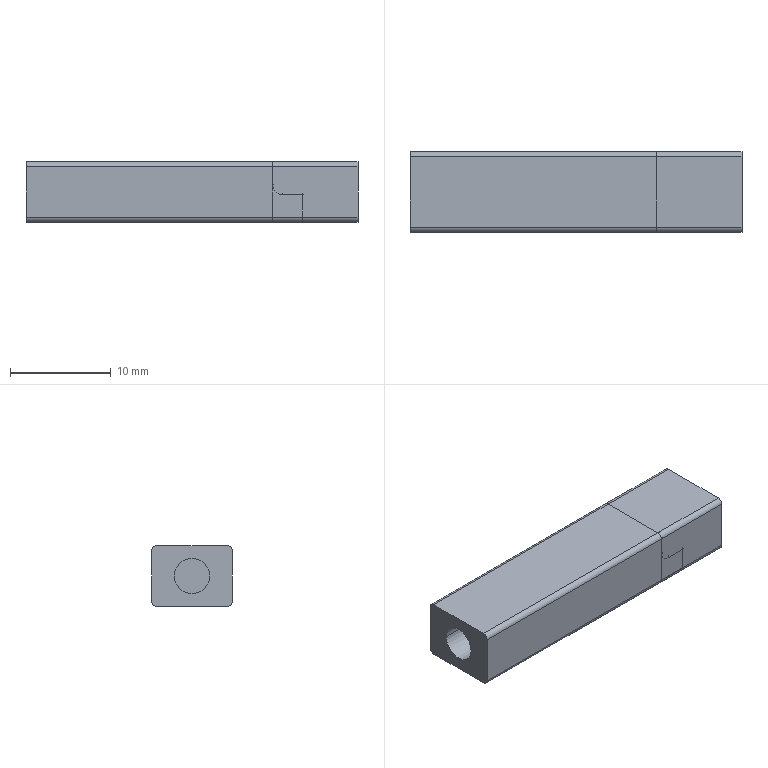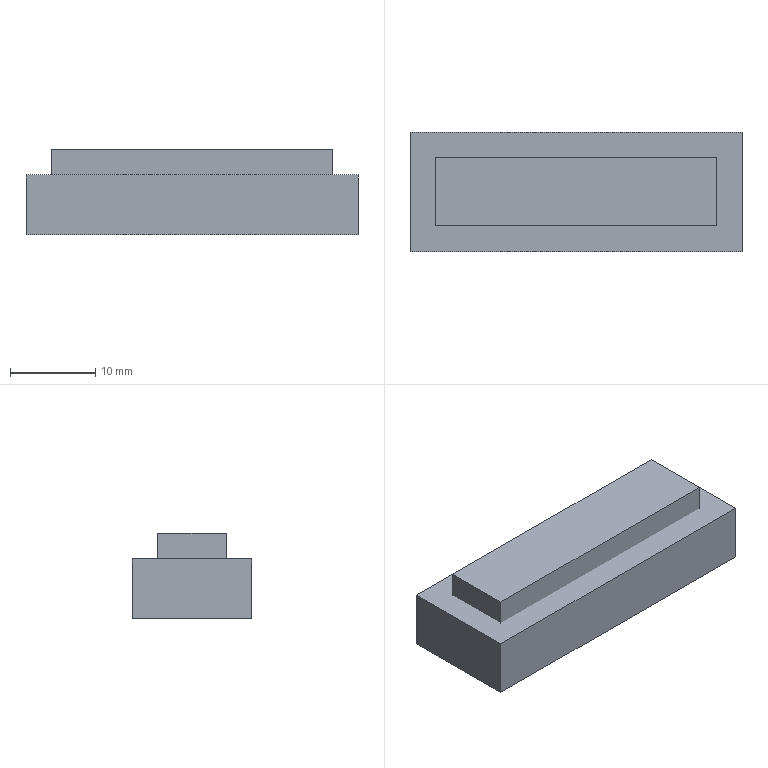CAM job | NX | 3+2 milling | part box 33 x 8 x 6 mm | stock box 39 x 14 x 10 mm
Tools:
number,name,description,diameter,corner_radius,flute_length,length,flutes
1,D63,Milling Tool-5 Parameters,63.0,0.0,50.0,75.0,2
9,D10,Milling Tool-5 Parameters,10.0,0.0,50.0,75.0,2
10,D10JING,Milling Tool-5 Parameters,10.0,0.0,50.0,75.0,2
8,D6R0.5,Milling Tool-5 Parameters,6.0,0.5,50.0,75.0,2
12,D2,Milling Tool-5 Parameters,2.0,0.0,50.0,75.0,2
4,D4,Milling Tool-5 Parameters,4.0,0.0,50.0,75.0,2
2,D4A45,Milling Tool-5 Parameters,4.0,0.0,2.0,2.0,2
11,D1,Milling Tool-5 Parameters,1.0,0.0,50.0,75.0,2
13,R0.5,Milling Tool-5 Parameters,1.0,0.5,50.0,75.0,2
Operations:
program,operation,operation_type,tool,method,geometry_group,spindle_rpm,surface_speed,feed_per_tooth,feed_cut,feed_plunge,cut_length_mm,path_length_mm,cut_time_min,machine_time_min
1,FLOOR_WALL,VolumeBased25DMillingOperation,D63,METHOD,A,6500.0,1286.0,0.0962,1250.0,100.0,114.0,168.0,0.0912,0.0966
1,ZLEVEL_PROFILE,ZLevelMilling,D10,METHOD,A,9500.0,298.0,0.1579,3000.0,1000.0,790.848,853.848,0.2955,0.3018
1,ZLEVEL_PROFILE_COPY_COPY,ZLevelMilling,D10JING,METHOD,A,9500.0,119.0,0.0632,1200.0,1000.0,121.754,190.754,0.1021,0.109
1,ZLEVEL_PROFILE_COPY_1,ZLevelMilling,D6R0.5,METHOD,A,9500.0,179.0,0.1579,3000.0,1000.0,1679.087,1811.412,0.5637,0.5769
2,FLOOR_WALL_COPY,VolumeBased25DMillingOperation,D63,METHOD,B,6500.0,1286.0,0.0962,1250.0,100.0,432.0,942.001,0.3456,0.3966
2,ZLEVEL_PROFILE_COPY_1_COPY,ZLevelMilling,D6R0.5,METHOD,B,9500.0,179.0,0.1579,3000.0,1000.0,1679.218,1811.504,0.5638,0.577
3,HOLE_MILLING,CylinderMilling,D2,METHOD,C,9500.0,59.0,0.0579,1100.0,100.0,501.981,571.481,0.4563,0.4633
3,ZLEVEL_PROFILE_1_COPY_1_COPY,ZLevelMilling,D4A45,METHOD,C,9500.0,179.0,0.0526,1000.0,100.0,45.673,170.24,0.0457,0.0581
4,CAVITY_MILL_COPY,CavityMilling,D4,METHOD,D,9500.0,119.0,0.1053,2000.0,1000.0,923.258,1062.641,0.4929,0.5068
4,ZLEVEL_PROFILE_COPY_COPY_COPY,ZLevelMilling,D4,METHOD,D,9500.0,119.0,0.0632,1200.0,1000.0,24.331,96.331,0.0207,0.0279
4,FLOOR_WALL_1,VolumeBased25DMillingOperation,D4,METHOD,D,9500.0,119.0,0.0526,1000.0,100.0,19.066,92.066,0.0191,0.0264
4,CAVITY_MILL_COPY_COPY,CavityMilling,D2,METHOD,D,9500.0,59.0,0.0526,1000.0,1000.0,176.406,431.235,0.1764,0.2019
4,ZLEVEL_PROFILE_COPY_1_COPY_COPY,ZLevelMilling,D2,METHOD,D,9500.0,59.0,0.0789,1500.0,1000.0,214.849,287.399,0.1439,0.1512
4,ZLEVEL_PROFILE_COPY_1_COPY_COPY_COPY_1,ZLevelMilling,D2,METHOD,D,9500.0,59.0,0.0789,1500.0,1000.0,266.624,340.134,0.1784,0.1858
4,FLOOR_WALL_1_COPY,VolumeBased25DMillingOperation,D2,METHOD,D,9500.0,119.0,0.0526,1000.0,100.0,45.718,189.039,0.0457,0.06
4,CAVITY_MILL_COPY_COPY_COPY,CavityMilling,D1,METHOD,D,9500.0,59.0,0.0526,1000.0,1000.0,464.409,744.399,0.4644,0.4924
4,ZLEVEL_PROFILE_COPY,ZLevelMilling,R0.5,METHOD,D,9500.0,29.0,0.1053,2000.0,1000.0,2070.043,2195.643,1.064,1.076
4,ZLEVEL_PROFILE_COPY_1_COPY_COPY_COPY,ZLevelMilling,R0.5,METHOD,D,9500.0,59.0,0.0789,1500.0,1000.0,956.199,1024.706,0.6381,0.6449